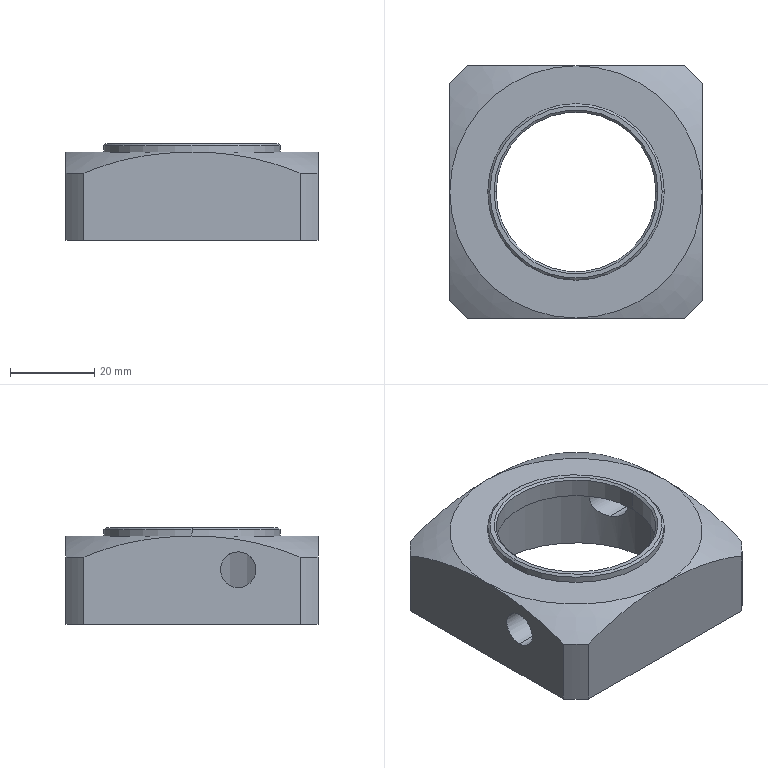Part | STEP file | B-PRF60 connecting plate, standard, tailstock type_1 | 1 solid | 46 faces | box 60 x 60 x 23 mm | volume 34147 mm3 | cylinder 22 | cone 12 | plane 8 | spline 4 | commonest cylinder face diameters 3.3 x8 8.5 x4 79 x4 38 x2 42 x2 50 x2